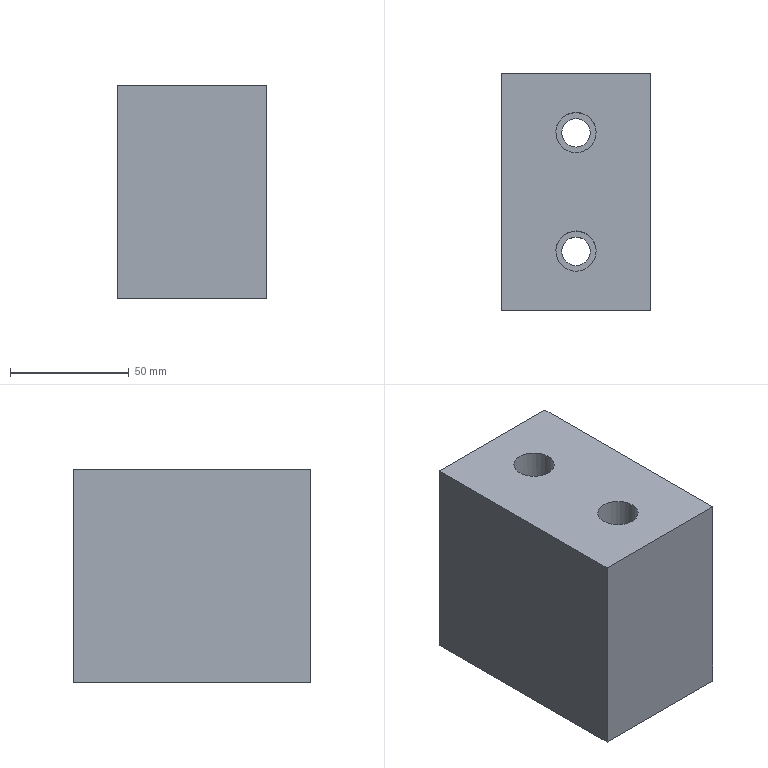Part | NX | features solid 2 | 1 solid | 12 faces | box 63 x 100 x 90 mm | volume 530699 mm3 | plane 8 | cylinder 4 | commonest cylinder face diameters 12 x2 17 x2
STEP:
#1=CARTESIAN_POINT('',(-1276.5,815.,-125.));
#2=VERTEX_POINT('',#1);
#3=CARTESIAN_POINT('',(-1276.5,815.,-35.));
#4=VERTEX_POINT('',#3);
#5=CARTESIAN_POINT('',(-1276.5,815.,-125.));
#6=DIRECTION('',(0.,0.,-1.));
#7=VECTOR('',#6,1000.);
#8=LINE('',#5,#7);
#9=EDGE_CURVE('',#2,#4,#8,.F.);
#10=ORIENTED_EDGE('',*,*,#9,.F.);
#11=CARTESIAN_POINT('',(-1276.5,715.,-125.));
#12=VERTEX_POINT('',#11);
#13=CARTESIAN_POINT('',(-1276.5,815.,-125.));
#14=DIRECTION('',(0.,-1.,0.));
#15=VECTOR('',#14,1000.);
#16=LINE('',#13,#15);
#17=EDGE_CURVE('',#2,#12,#16,.T.);
#18=ORIENTED_EDGE('',*,*,#17,.T.);
#19=CARTESIAN_POINT('',(-1276.5,715.,-35.));
#20=VERTEX_POINT('',#19);
#21=CARTESIAN_POINT('',(-1276.5,715.,-125.));
#22=DIRECTION('',(0.,0.,1.));
#23=VECTOR('',#22,1000.);
#24=LINE('',#21,#23);
#25=EDGE_CURVE('',#12,#20,#24,.T.);
#26=ORIENTED_EDGE('',*,*,#25,.T.);
#27=CARTESIAN_POINT('',(-1276.5,815.,-35.));
#28=DIRECTION('',(0.,-1.,0.));
#29=VECTOR('',#28,1000.);
#30=LINE('',#27,#29);
#31=EDGE_CURVE('',#4,#20,#30,.T.);
#32=ORIENTED_EDGE('',*,*,#31,.F.);
#33=EDGE_LOOP('',(#10,#18,#26,#32));
#34=FACE_BOUND('',#33,.T.);
#35=CARTESIAN_POINT('',(-1276.5,815.,-125.));
#36=DIRECTION('',(-1.,0.,0.));
#37=DIRECTION('',(0.,-1.,0.));
#38=AXIS2_PLACEMENT_3D('',#35,#36,#37);
#39=PLANE('',#38);
#40=ADVANCED_FACE('',(#34),#39,.T.);
#41=ORIENTED_EDGE('',*,*,#25,.F.);
#42=CARTESIAN_POINT('',(-1213.5,715.,-125.));
#43=VERTEX_POINT('',#42);
#44=CARTESIAN_POINT('',(-1275.,715.,-125.));
#45=DIRECTION('',(1.,0.,0.));
#46=VECTOR('',#45,1000.);
#47=LINE('',#44,#46);
#48=EDGE_CURVE('',#12,#43,#47,.T.);
#49=ORIENTED_EDGE('',*,*,#48,.T.);
#50=CARTESIAN_POINT('',(-1213.5,715.,-35.));
#51=VERTEX_POINT('',#50);
#52=CARTESIAN_POINT('',(-1213.5,715.,-125.));
#53=DIRECTION('',(0.,0.,-1.));
#54=VECTOR('',#53,1000.);
#55=LINE('',#52,#54);
#56=EDGE_CURVE('',#43,#51,#55,.F.);
#57=ORIENTED_EDGE('',*,*,#56,.T.);
#58=CARTESIAN_POINT('',(-1275.,715.,-35.));
#59=DIRECTION('',(1.,0.,0.));
#60=VECTOR('',#59,1000.);
#61=LINE('',#58,#60);
#62=EDGE_CURVE('',#20,#51,#61,.T.);
#63=ORIENTED_EDGE('',*,*,#62,.F.);
#64=EDGE_LOOP('',(#41,#49,#57,#63));
#65=FACE_BOUND('',#64,.T.);
#66=CARTESIAN_POINT('',(-1275.,715.,-125.));
#67=DIRECTION('',(0.,-1.,0.));
#68=DIRECTION('',(1.,0.,0.));
#69=AXIS2_PLACEMENT_3D('',#66,#67,#68);
#70=PLANE('',#69);
#71=ADVANCED_FACE('',(#65),#70,.T.);
#72=ORIENTED_EDGE('',*,*,#56,.F.);
#73=CARTESIAN_POINT('',(-1213.5,815.,-125.));
#74=VERTEX_POINT('',#73);
#75=CARTESIAN_POINT('',(-1213.5,815.,-125.));
#76=DIRECTION('',(0.,1.,0.));
#77=VECTOR('',#76,1000.);
#78=LINE('',#75,#77);
#79=EDGE_CURVE('',#74,#43,#78,.F.);
#80=ORIENTED_EDGE('',*,*,#79,.F.);
#81=CARTESIAN_POINT('',(-1213.5,815.,-35.));
#82=VERTEX_POINT('',#81);
#83=CARTESIAN_POINT('',(-1213.5,815.,-125.));
#84=DIRECTION('',(0.,0.,1.));
#85=VECTOR('',#84,1000.);
#86=LINE('',#83,#85);
#87=EDGE_CURVE('',#74,#82,#86,.T.);
#88=ORIENTED_EDGE('',*,*,#87,.T.);
#89=CARTESIAN_POINT('',(-1213.5,815.,-35.));
#90=DIRECTION('',(0.,1.,0.));
#91=VECTOR('',#90,1000.);
#92=LINE('',#89,#91);
#93=EDGE_CURVE('',#82,#51,#92,.F.);
#94=ORIENTED_EDGE('',*,*,#93,.T.);
#95=EDGE_LOOP('',(#72,#80,#88,#94));
#96=FACE_BOUND('',#95,.T.);
#97=CARTESIAN_POINT('',(-1213.5,815.,-125.));
#98=DIRECTION('',(-1.,0.,0.));
#99=DIRECTION('',(0.,-1.,0.));
#100=AXIS2_PLACEMENT_3D('',#97,#98,#99);
#101=PLANE('',#100);
#102=ADVANCED_FACE('',(#96),#101,.F.);
#103=CARTESIAN_POINT('',(-1275.,815.,-125.));
#104=DIRECTION('',(1.,0.,0.));
#105=VECTOR('',#104,1000.);
#106=LINE('',#103,#105);
#107=EDGE_CURVE('',#2,#74,#106,.T.);
#108=ORIENTED_EDGE('',*,*,#107,.F.);
#109=ORIENTED_EDGE('',*,*,#9,.T.);
#110=CARTESIAN_POINT('',(-1275.,815.,-35.));
#111=DIRECTION('',(-1.,0.,0.));
#112=VECTOR('',#111,1000.);
#113=LINE('',#110,#112);
#114=EDGE_CURVE('',#4,#82,#113,.F.);
#115=ORIENTED_EDGE('',*,*,#114,.T.);
#116=ORIENTED_EDGE('',*,*,#87,.F.);
#117=EDGE_LOOP('',(#108,#109,#115,#116));
#118=FACE_BOUND('',#117,.T.);
#119=CARTESIAN_POINT('',(-1275.,815.,-125.));
#120=DIRECTION('',(0.,-1.,0.));
#121=DIRECTION('',(1.,0.,0.));
#122=AXIS2_PLACEMENT_3D('',#119,#120,#121);
#123=PLANE('',#122);
#124=ADVANCED_FACE('',(#118),#123,.F.);
#125=CARTESIAN_POINT('',(-1236.5,740.,-35.));
#126=VERTEX_POINT('',#125);
#127=CARTESIAN_POINT('',(-1245.,740.,-35.));
#128=DIRECTION('',(0.,0.,1.));
#129=DIRECTION('',(1.,0.,0.));
#130=AXIS2_PLACEMENT_3D('',#127,#128,#129);
#131=CIRCLE('',#130,8.5);
#132=EDGE_CURVE('',#126,#126,#131,.F.);
#133=ORIENTED_EDGE('',*,*,#132,.T.);
#134=EDGE_LOOP('',(#133));
#135=FACE_BOUND('',#134,.T.);
#136=CARTESIAN_POINT('',(-1236.5,790.,-35.));
#137=VERTEX_POINT('',#136);
#138=CARTESIAN_POINT('',(-1245.,790.,-35.));
#139=DIRECTION('',(0.,0.,1.));
#140=DIRECTION('',(1.,0.,0.));
#141=AXIS2_PLACEMENT_3D('',#138,#139,#140);
#142=CIRCLE('',#141,8.5);
#143=EDGE_CURVE('',#137,#137,#142,.F.);
#144=ORIENTED_EDGE('',*,*,#143,.T.);
#145=EDGE_LOOP('',(#144));
#146=FACE_BOUND('',#145,.T.);
#147=ORIENTED_EDGE('',*,*,#93,.F.);
#148=ORIENTED_EDGE('',*,*,#114,.F.);
#149=ORIENTED_EDGE('',*,*,#31,.T.);
#150=ORIENTED_EDGE('',*,*,#62,.T.);
#151=EDGE_LOOP('',(#147,#148,#149,#150));
#152=FACE_BOUND('',#151,.T.);
#153=CARTESIAN_POINT('',(-1275.,815.,-35.));
#154=DIRECTION('',(0.,0.,1.));
#155=DIRECTION('',(0.,-1.,0.));
#156=AXIS2_PLACEMENT_3D('',#153,#154,#155);
#157=PLANE('',#156);
#158=ADVANCED_FACE('',(#135,#146,#152),#157,.T.);
#159=CARTESIAN_POINT('',(-1245.,734.,-125.));
#160=VERTEX_POINT('',#159);
#161=CARTESIAN_POINT('',(-1245.,740.,-125.));
#162=DIRECTION('',(0.,0.,1.));
#163=DIRECTION('',(0.,-1.,0.));
#164=AXIS2_PLACEMENT_3D('',#161,#162,#163);
#165=CIRCLE('',#164,6.);
#166=EDGE_CURVE('',#160,#160,#165,.T.);
#167=ORIENTED_EDGE('',*,*,#166,.T.);
#168=EDGE_LOOP('',(#167));
#169=FACE_BOUND('',#168,.T.);
#170=CARTESIAN_POINT('',(-1245.,784.,-125.));
#171=VERTEX_POINT('',#170);
#172=CARTESIAN_POINT('',(-1245.,790.,-125.));
#173=DIRECTION('',(0.,0.,1.));
#174=DIRECTION('',(0.,-1.,0.));
#175=AXIS2_PLACEMENT_3D('',#172,#173,#174);
#176=CIRCLE('',#175,6.);
#177=EDGE_CURVE('',#171,#171,#176,.T.);
#178=ORIENTED_EDGE('',*,*,#177,.T.);
#179=EDGE_LOOP('',(#178));
#180=FACE_BOUND('',#179,.T.);
#181=ORIENTED_EDGE('',*,*,#79,.T.);
#182=ORIENTED_EDGE('',*,*,#48,.F.);
#183=ORIENTED_EDGE('',*,*,#17,.F.);
#184=ORIENTED_EDGE('',*,*,#107,.T.);
#185=EDGE_LOOP('',(#181,#182,#183,#184));
#186=FACE_BOUND('',#185,.T.);
#187=CARTESIAN_POINT('',(-1275.,815.,-125.));
#188=DIRECTION('',(0.,0.,1.));
#189=DIRECTION('',(0.,-1.,0.));
#190=AXIS2_PLACEMENT_3D('',#187,#188,#189);
#191=PLANE('',#190);
#192=ADVANCED_FACE('',(#169,#180,#186),#191,.F.);
#193=CARTESIAN_POINT('',(-1245.,796.,-105.));
#194=VERTEX_POINT('',#193);
#195=CARTESIAN_POINT('',(-1245.,790.,-105.));
#196=DIRECTION('',(0.,0.,-1.));
#197=DIRECTION('',(0.,1.,0.));
#198=AXIS2_PLACEMENT_3D('',#195,#196,#197);
#199=CIRCLE('',#198,6.);
#200=EDGE_CURVE('',#194,#194,#199,.T.);
#201=ORIENTED_EDGE('',*,*,#200,.T.);
#202=EDGE_LOOP('',(#201));
#203=FACE_BOUND('',#202,.T.);
#204=CARTESIAN_POINT('',(-1245.,798.5,-105.));
#205=VERTEX_POINT('',#204);
#206=CARTESIAN_POINT('',(-1245.,790.,-105.));
#207=DIRECTION('',(0.,0.,-1.));
#208=DIRECTION('',(0.,1.,0.));
#209=AXIS2_PLACEMENT_3D('',#206,#207,#208);
#210=CIRCLE('',#209,8.5);
#211=EDGE_CURVE('',#205,#205,#210,.T.);
#212=ORIENTED_EDGE('',*,*,#211,.F.);
#213=EDGE_LOOP('',(#212));
#214=FACE_BOUND('',#213,.T.);
#215=CARTESIAN_POINT('',(-1245.,790.,-105.));
#216=DIRECTION('',(0.,0.,-1.));
#217=DIRECTION('',(0.,1.,0.));
#218=AXIS2_PLACEMENT_3D('',#215,#216,#217);
#219=PLANE('',#218);
#220=ADVANCED_FACE('',(#203,#214),#219,.F.);
#221=ORIENTED_EDGE('',*,*,#211,.T.);
#222=EDGE_LOOP('',(#221));
#223=FACE_BOUND('',#222,.T.);
#224=ORIENTED_EDGE('',*,*,#143,.F.);
#225=EDGE_LOOP('',(#224));
#226=FACE_BOUND('',#225,.T.);
#227=CARTESIAN_POINT('',(-1245.,790.,-15.));
#228=DIRECTION('',(0.,0.,-1.));
#229=DIRECTION('',(0.,1.,0.));
#230=AXIS2_PLACEMENT_3D('',#227,#228,#229);
#231=CYLINDRICAL_SURFACE('',#230,8.5);
#232=ADVANCED_FACE('',(#223,#226),#231,.F.);
#233=CARTESIAN_POINT('',(-1245.,746.,-105.));
#234=VERTEX_POINT('',#233);
#235=CARTESIAN_POINT('',(-1245.,740.,-105.));
#236=DIRECTION('',(0.,0.,-1.));
#237=DIRECTION('',(0.,1.,0.));
#238=AXIS2_PLACEMENT_3D('',#235,#236,#237);
#239=CIRCLE('',#238,6.);
#240=EDGE_CURVE('',#234,#234,#239,.T.);
#241=ORIENTED_EDGE('',*,*,#240,.T.);
#242=EDGE_LOOP('',(#241));
#243=FACE_BOUND('',#242,.T.);
#244=CARTESIAN_POINT('',(-1245.,748.5,-105.));
#245=VERTEX_POINT('',#244);
#246=CARTESIAN_POINT('',(-1245.,740.,-105.));
#247=DIRECTION('',(0.,0.,-1.));
#248=DIRECTION('',(0.,1.,0.));
#249=AXIS2_PLACEMENT_3D('',#246,#247,#248);
#250=CIRCLE('',#249,8.5);
#251=EDGE_CURVE('',#245,#245,#250,.T.);
#252=ORIENTED_EDGE('',*,*,#251,.F.);
#253=EDGE_LOOP('',(#252));
#254=FACE_BOUND('',#253,.T.);
#255=CARTESIAN_POINT('',(-1245.,740.,-105.));
#256=DIRECTION('',(0.,0.,-1.));
#257=DIRECTION('',(0.,1.,0.));
#258=AXIS2_PLACEMENT_3D('',#255,#256,#257);
#259=PLANE('',#258);
#260=ADVANCED_FACE('',(#243,#254),#259,.F.);
#261=ORIENTED_EDGE('',*,*,#251,.T.);
#262=EDGE_LOOP('',(#261));
#263=FACE_BOUND('',#262,.T.);
#264=ORIENTED_EDGE('',*,*,#132,.F.);
#265=EDGE_LOOP('',(#264));
#266=FACE_BOUND('',#265,.T.);
#267=CARTESIAN_POINT('',(-1245.,740.,-15.));
#268=DIRECTION('',(0.,0.,-1.));
#269=DIRECTION('',(0.,1.,0.));
#270=AXIS2_PLACEMENT_3D('',#267,#268,#269);
#271=CYLINDRICAL_SURFACE('',#270,8.5);
#272=ADVANCED_FACE('',(#263,#266),#271,.F.);
#273=ORIENTED_EDGE('',*,*,#200,.F.);
#274=EDGE_LOOP('',(#273));
#275=FACE_BOUND('',#274,.T.);
#276=ORIENTED_EDGE('',*,*,#177,.F.);
#277=EDGE_LOOP('',(#276));
#278=FACE_BOUND('',#277,.T.);
#279=CARTESIAN_POINT('',(-1245.,790.,-105.));
#280=DIRECTION('',(0.,0.,-1.));
#281=DIRECTION('',(0.,1.,0.));
#282=AXIS2_PLACEMENT_3D('',#279,#280,#281);
#283=CYLINDRICAL_SURFACE('',#282,6.);
#284=ADVANCED_FACE('',(#275,#278),#283,.F.);
#285=ORIENTED_EDGE('',*,*,#240,.F.);
#286=EDGE_LOOP('',(#285));
#287=FACE_BOUND('',#286,.T.);
#288=ORIENTED_EDGE('',*,*,#166,.F.);
#289=EDGE_LOOP('',(#288));
#290=FACE_BOUND('',#289,.T.);
#291=CARTESIAN_POINT('',(-1245.,740.,-105.));
#292=DIRECTION('',(0.,0.,-1.));
#293=DIRECTION('',(0.,1.,0.));
#294=AXIS2_PLACEMENT_3D('',#291,#292,#293);
#295=CYLINDRICAL_SURFACE('',#294,6.);
#296=ADVANCED_FACE('',(#287,#290),#295,.F.);
#297=CLOSED_SHELL('',(#40,#71,#102,#124,#158,#192,#220,#232,#260,#272,#284,#296));
#298=MANIFOLD_SOLID_BREP('',#297);
#299=(LENGTH_UNIT()NAMED_UNIT(*)SI_UNIT(.MILLI.,.METRE.));
#300=UNCERTAINTY_MEASURE_WITH_UNIT(LENGTH_MEASURE(0.00001),#299,'','');
#301=(NAMED_UNIT(*)PLANE_ANGLE_UNIT()SI_UNIT($,.RADIAN.));
#302=(NAMED_UNIT(*)SI_UNIT($,.STERADIAN.)SOLID_ANGLE_UNIT());
#303=(GEOMETRIC_REPRESENTATION_CONTEXT(3)GLOBAL_UNCERTAINTY_ASSIGNED_CONTEXT((#300))GLOBAL_UNIT_ASSIGNED_CONTEXT((#299,#301,#302))REPRESENTATION_CONTEXT('',''));
#304=ADVANCED_BREP_SHAPE_REPRESENTATION('',(#298),#303);